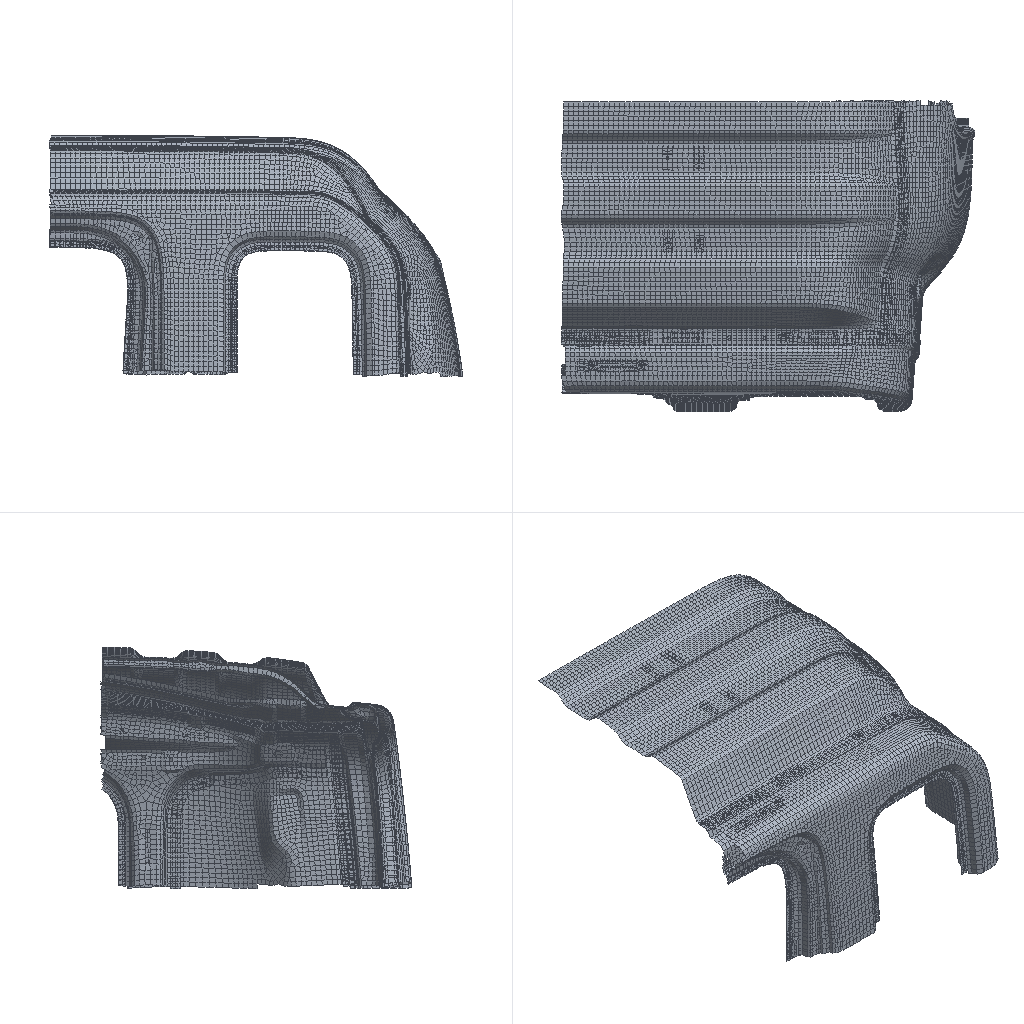Simulation study | nastran
Set-up summary:
category,name,step,type,value,unit,region
solver,nx_nastran
units,not stated in the deck,,not stated
analysis,deck,,static,static
analysis,solution,,SOL,101
load_step,SUBCASE 2,2,SUBCASE,SPC=2 LOAD=3
load_step,SUBCASE 3,3,SUBCASE,SPC=2 LOAD=4
load_step,SUBCASE 4,4,SUBCASE,SPC=2 LOAD=5
load_step,requested,,,3
mesh,nodes,,,18709
mesh,elements,,,17229
element_type,CHEXA,,unverified,95
element_type,CQUAD4,,shell,16781
element_type,CTRIA3,,shell,448
load,load commands in deck,,count,3
bc,support commands in deck,,count,589
check,setup vs results,,match,"every grid point's frame and coordinates and every element id; grid points of CHEXA, CQUAD4, CTRIA3 elements"
Nastran input file, long lists of numbers shortened:
$$------------------------------------------------------------------------------$
$$                                                                              $
$$ NASTRAN Input Deck Generated by HyperMesh Version  :10.0buil                 $
$$ Generated using HyperMesh-Nastran Template Version : 10.0build60
$$                                                                              $
$$   Template:  general                                                         $
$$                                                                              $
$$------------------------------------------------------------------------------$
$$------------------------------------------------------------------------------$
$$                      Executive Control Cards                                 $
$$------------------------------------------------------------------------------$
SOL 101
CEND
$$------------------------------------------------------------------------------$
$$                      Case Control Cards                                      $
$$------------------------------------------------------------------------------$
  DISPLACEMENT = ALL
  ESE = ALL
$
$HMNAME LOADSTEP               2"fx"
SUBCASE       2
  LABEL=   fx
  SPC =        2
  LOAD =        3
$
$HMNAME LOADSTEP               3"fy"
SUBCASE       3
  LABEL=   fy
  SPC =        2
  LOAD =        4
$
$HMNAME LOADSTEP               4"fz"
SUBCASE       4
  LABEL=   fz
  SPC =        2
  LOAD =        5
$$------------------------------------------------------------------------------$
$$                      Bulk Data Cards                                         $
$$------------------------------------------------------------------------------$
BEGIN BULK
PARAM,POST,-1
$$
$$  GRID Data
$$
GRID          67        5.69744 -963.1871605.389
GRID          69        25.16258-962.9811605.619
$ (18707 more lines like these left out)
$$
$$  SPOINT Data
$$
$$
$$------------------------------------------------------------------------------$
$$             Group Definitions                                                $
$$------------------------------------------------------------------------------$
$$
$$ RBE2 Elements - Multiple dependent nodes
$$
RBE2     101300284098578  123456  615860  615861  615864  615865  615866+
+         615867  615868  615869  615870  615871  615872  615873  619696+
+         619697  619698  620859  620860  620861  620874  620875  620876+
+         620966  620967  620968  620995  620996  621455  621456  621457+
+         621458  621459  621506  621555  621586  621610  621611  621634+
+         623382  623383  623384  624034  624035  624114  624115  624144+
+         624145  624164  624165  624242  624243  624449  624450  624453+
+         624454  624455  624456  624457  624458  624465  624466  624469+
+         624470  624473  624474  624475  624476  624620  624621  624742+
+         624743  624772  624773  624886  624887  624962  624963  625075+
+         625076  625083  625084  625106  625110  625156  625157  625872+
+         625874  625889  629153  629154  629188  629189  629227  629229+
+         632251  632252  632256  632257  632258  632533  632534  632540+
+         632541  632542  632543  632544  632546  632547  632549  632550+
+         633449  633450  633451  633452  633453  633454  633455  633456+
+         633457  633458  633459  633460  633461  633462  633463  633464+
+         633465  633466  633467  633468  633469  634976  634977  634978+
+         634984  634985  635013  635015  635017  635050  635051  635093+
+         635094  635095  635138  635139  635140  635187  635188  635189+
+         635197  635198  635199  635236  635240  635248  635252  635256+
+         635698  635699  635700  635707  635708  635709  636086  636087+
+         636090  636221  636222  636225  636226  636265  636266  636282+
+         636283  636313  636314  636315  636316  636317  636318  636345+
+         636346  636355  636356  636361  636362  636367  636368  636624+
+         636625  636653  636654  636669  636674  636784  636785  636920+
+         636921  636922  636923  636925  637560  637561  637562  637587+
+         637588  637589  637613  637614  637615  637645  637646  637647+
+         637661  637662  637663  637675  637676  637677  637703  637704+
+         637705  637710  637711  637712  638987  638988  639142  639143+
+         639298  639315  639600  639601  639606  639607  640059  640060+
+         640061  640071  640072  640073  640559  640560  640561  640579+
+         640591  640593  642212  642678  642679  642682  642683  642684+
+         642685  642707  642712  642713  642715  642717  642718  642720+
+         642721  642723  642726  642728  642732  642862  642863  643164+
+         643166  643167  643177  643178  643179  645382  645411  645412+
+         645413  645439  645440 3753700 3753701 3753759 3753760 3753761+
+        3753771 3753772 3753869 3753870 3753871 3753904 3753907 3753909+
+        3753990 3753991 3753992 3754005 3754006 3754007 3754008 3754009+
+        3754010 3754049 3754050 3754061 3754062 3754091 3754092 3754138+
+        3754139 3754179 3754180 3754187 3754188 3754231 3754232 3754233+
+        3754234 3754347 3754348 3754375 3754376 3754401 3754402 3754431+
+        3754432 3754433 3754434 3754435 3754445 3754446 3754447 3754449+
+        3754450 3754455 3754456 3754478 3754479 3754498 3754499 3754520+
+        3754521 3754587
$
$HMMOVE 84022693
$        1013002
$
$
$  RBE3 Elements
$
RBE3      327723         3756869  1234560.591263     123  6251265.44E-04+
+            123  6251033.75E-04     123  6251040.407818     123  625058
RBE3      327724         3756870  1234560.005572     123  6251000.175196+
+            123  6251010.793976     123  6251260.025254     123  625125
$ (1516 more lines like these left out)
$
$HMMOVE 57005012
$         327723THRU      327726  327728THRU      327735  327737THRU      327744
$         327746THRU      327753  327755THRU      327762  327764THRU      327771
$ (41 more lines like these left out)
CTRIA3    145456       1   58012   57983   57984
CTRIA3    145466       1   58018   58019   58016
$ (446 more lines like these left out)
$
$HMMOVE       14
$         145456  145466  145470  146282  146292  146300  146309THRU      146310
$         146354  146362  146465  146535  146580  146635  146684  146686  146706
$ (76 more lines like these left out)
CQUAD4    189186       1   59396   59395   65859   65858
CQUAD4    189187       1   59397   59396   65858   65857
$ (16779 more lines like these left out)
$
$HMMOVE       14
$         189186THRU      189191  189212THRU      189222  190550THRU      190552
$         190862THRU      190879  195621  195623  195625  195646  195648  195658
$ (449 more lines like these left out)
CHEXA     327727      10 3756869 3756870 3756871 3756872 3756873 3756874+
+        3756875 3756876
CHEXA     327736      10 3756878 3756881 3756880 3756879 3756882 3756885+
+        3756884 3756883
$ (186 more lines like these left out)
$
$HMMOVE 57005011
$         327727  327736  327745  327754  327763  327772  328177  328186  328195
$         328204  328213  328222  328231  328240  328267  328276  328447  328456
$ (71 more lines like these left out)
PSHELL         1       10.8            1               1
$
$HMNAME PROP                   2"120" 4
$HWCOLOR PROP                  2       3
PSHELL         2       11.2            1               1
$
$HMNAME PROP                   5"150" 4
$HWCOLOR PROP                  5       3
PSHELL         5       11.5            1               1
$$
$$  PSOLID Data
$
$HMNAME PROP                  10"spot" 5
$HWCOLOR PROP                 10       3
PSOLID        10       1
$$
$$------------------------------------------------------------------------------$
$$                      Material Definition Cards                               $
$$------------------------------------------------------------------------------$
$$--------------------------------------------------------------
$$ HYPERMESH TAGS
$$--------------------------------------------------------------
$$BEGIN TAGS
$$END TAGS
$$
$$  MAT1 Data
$
$HMNAME MAT                    1"steel" "MAT1"
$HWCOLOR MAT                   1       3
MAT1           1210000.0        0.3     7.80E-09
$$
$$
$$
$$------------------------------------------------------------------------------$
$ (42 more lines like these left out)
SPC            2   54694  1234560.0
SPC            2   54641  1234560.0
SPC            2   53632  1234560.0
SPC            2   53551  1234560.0
$ (585 more lines like these left out)
$$
$$  FORCE Data
$$
FORCE          384098578       01.0     500.0   0.0     0.0
FORCE          484098578       01.0     0.0     500.0   0.0
FORCE          584098578       01.0     0.0     0.0     500.0
$HMASSEM      27       3 5600010
$HMASSEM_IDS          14      15
$HMASSEM 5700100       5 5700100
$HMASSEM_IDS    5700101057004010
$HMASSEM 5400100       7 sidebody_L
$HMASSEM_IDS    5400101054005010540070105400702054005020
$HMASSEM 5700101      11 New Assembly
$HMASSEM_IDS    5700501157005012
$HMASSEM_ASSEM_ID             27 5700100 5400100
$
ENDDATA
Results summary:
result,analysis,,,static
result,last_loadstep,,,3
result,primary field,,,displacements
result,max displacement,,,0.227,model units